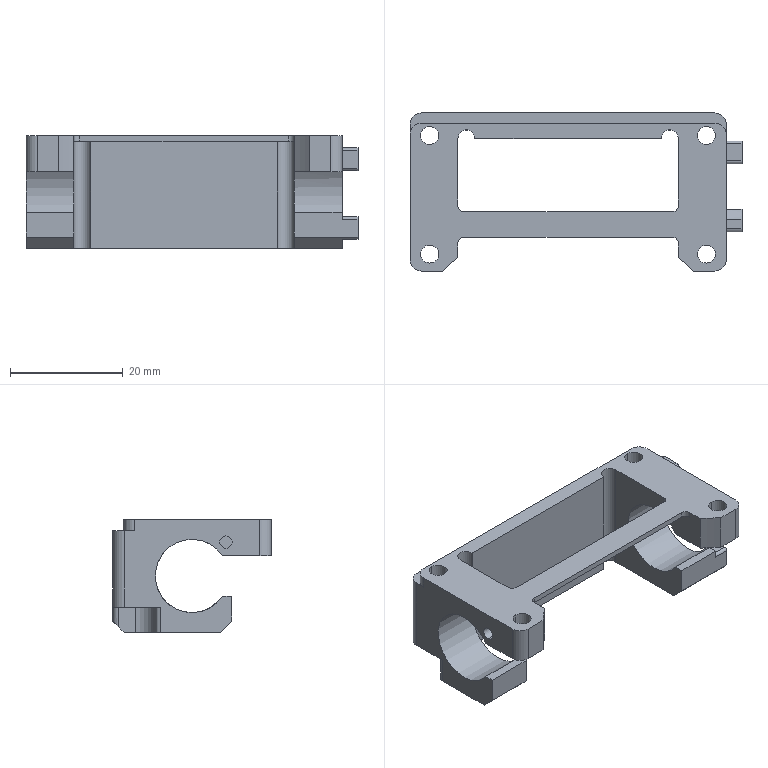Part | 1 solid | 87 faces | box 58.8 x 28 x 20 mm | volume 7876 mm3 | plane 44 | cylinder 43 | commonest cylinder face diameters 2 x8 3.2 x8 4 x6 1 x5 1.8 x4 2.2 x4